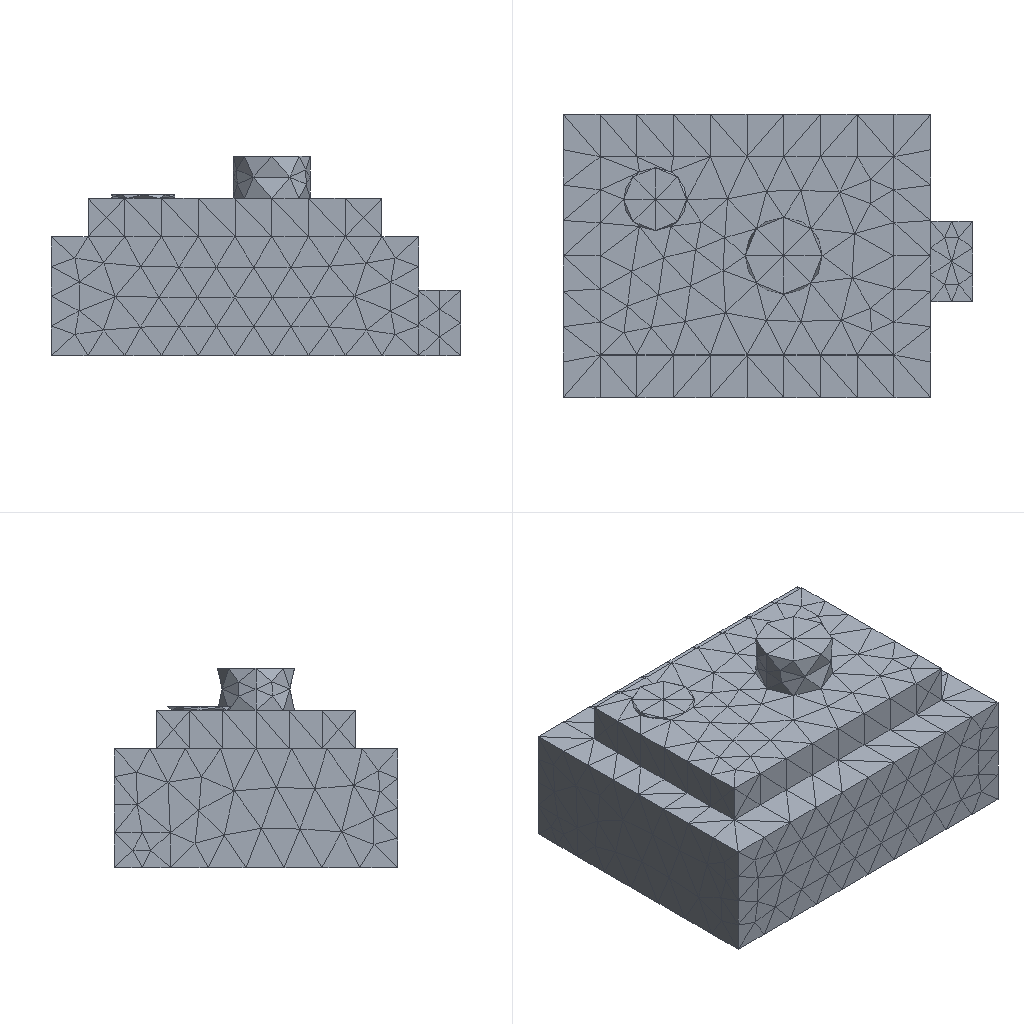Simulation study | ansys mapdl
Set-up summary:
category,name,step,type,value,unit,region
solver,ansys_mapdl
units,mm-N-s-tonne (MPa),,inferred,E=210000 density=
analysis,model,,static
mesh,nodes,,,5108
mesh,elements,,,3089
element_type,SOLID187,,,3089
material,mat 1,,E,210000
material,mat 1,,nu,0.3
load,,model,body load temp,,,all
load,,model,force,"1000 [dir=(0, 0, -1) n=146]",,node list
bc,,model,fixed,"[dofs=UX,UY,UZ n=5818]",,node list
Ansys APDL input file, long lists of numbers shortened:
/COM,ANSYS RELEASE 2026 R1           BUILD 26.1      UP20260202       09:09:22
/PREP7
/NOPR
/TITLE,2
ANTYPE, 0
*IF,_CDRDOFF,EQ,1,THEN     !if solid model was read in
_CDRDOFF=             !reset flag, numoffs already performed
*ELSE              !offset database for the following FE model
NUMOFF,NODE,     5108
NUMOFF,ELEM,     3089
NUMOFF,MAT ,        1
NUMOFF,TYPE,        1
*ENDIF
*SET,_RETURN ,  0.
*SET,_STATUS ,  0.
*SET,_UIQR   ,  146.
*SET,__FLOATPARAMETER__,  5108.
DOF,DELETE
ETBLOCK,        1,        1
(2i9,19a9)
        1      187        0        0        0        0        0        0        0        0        0        0        0        0        0        0        0        0        0        0        0
       -1
NBLOCK,6,SOLID,      5108,      5108
(3i9,6e21.13e3)
        1        0        0-3.6525000000000E+001 4.0500000000000E+001 1.0000000000000E+001
! (5107 more lines like these left out)
N,UNBL,LOC,       -1,
EBLOCK,19,SOLID,      3089,      3089
(19i10)
         1         1         1         1         0         0         0         0        10         0         1      1883      1884      1885      1886      2186      2187      2188      2189
! (6177 more lines like these left out)
        -1
MPTEMP,UNBL, 1, 1,  0.    ,
MPDATA,UNBL, 1,EX  ,       1, 1,  210000.000    ,
MPTEMP,UNBL, 1, 1,  0.    ,
MPDATA,UNBL, 1,NUXY,       1, 1, 0.3    ,
MPTEMP,UNBL, 1, 1,  0.    ,
MPDATA,UNBL, 1,PRXY,       1, 1, 0.3    ,
EXTOPT,ATTR,      0,      0,      0
EXTOPT,ESIZE,  0,  0.
EXTOPT,ACLEAR,      0
TREF,  0.
IRLF,  0
BFUNIF,TEMP,_TINY
ACEL,  0.    ,  0.    ,  0.
OMEGA,  0.    ,  0.    ,  0.
DOMEGA,  0.    ,  0.    ,  0.
CGLOC,  0.    ,  0.    ,  0.
CGOMEGA,  0.    ,  0.    ,  0.
DCGOMG,  0.    ,  0.    ,  0.
KUSE,     0
TIME,  0.
ALPHAD,  0.
BETAD,  0.
DMPRAT,  0.
DMPSTR,  0.
CRPLIM, 0.1    ,   0
CRPLIM,  0.    ,   1
NCNV,     0, 1.000000000E+12,     0,  0.    ,  0.
NEQIT,     0
ERESX,DEFA
DBLOCK,      5818
(i9,a6,2(pg16.9))
        1  UX    0.00000000      0.00000000
! (5817 more lines like these left out)
       -1
FBLOCK,       146
(i9,a6,2(pg16.9))
      890  FZ   -6.84931507      0.00000000
! (145 more lines like these left out)
       -1
/GO
FINISH
Results summary:
result,analysis_type_db,,,static,unstated
result,n_sets,,,1,unstated
result,load_steps[0].set,load_step=1,,1,unstated
result,load_steps[0].substep,load_step=1,,1,unstated
result,load_steps[0].time,load_step=1,,1,unstated
result,load_steps[0].freq,load_step=1,,1,unstated
result,load_steps[0].max_usum,load_step=1,,0.0003182,unstated
result,load_steps[0].max_seqv,load_step=1,,3.563,unstated
result,load_steps[0].reaction_sum.FX,load_step=1,,-1.88688e-11,unstated
result,load_steps[0].reaction_sum.FY,load_step=1,,-9.34313e-12,unstated
result,load_steps[0].reaction_sum.FZ,load_step=1,,1000,unstated
result,load_steps[0].reaction_sum.MX,load_step=1,,0,unstated
result,load_steps[0].reaction_sum.MY,load_step=1,,0,unstated
result,load_steps[0].reaction_sum.MZ,load_step=1,,0,unstated
result,convergence,,,results present for all listed sets,unstated